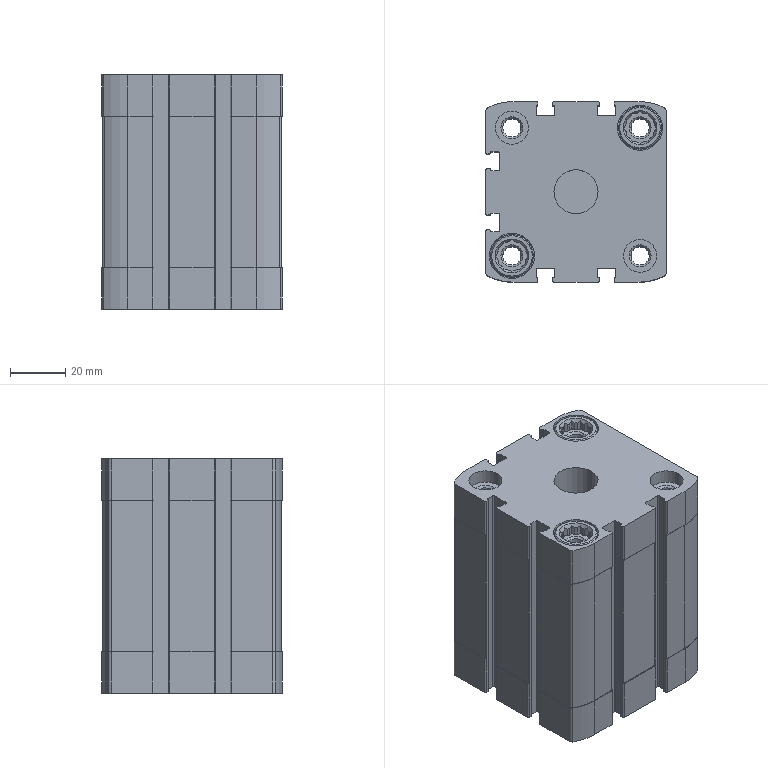Part | SolidWorks | features BaseBody 1 | 1 solid | 449 faces | box 65.5 x 65.5 x 85 mm | volume 218537 mm3 | plane 211 | cylinder 202 | cone 36 | commonest cylinder face diameters 0.8 x48 10.6 x48 0.4 x24 6.647 x16 12 x10 2.7 x8